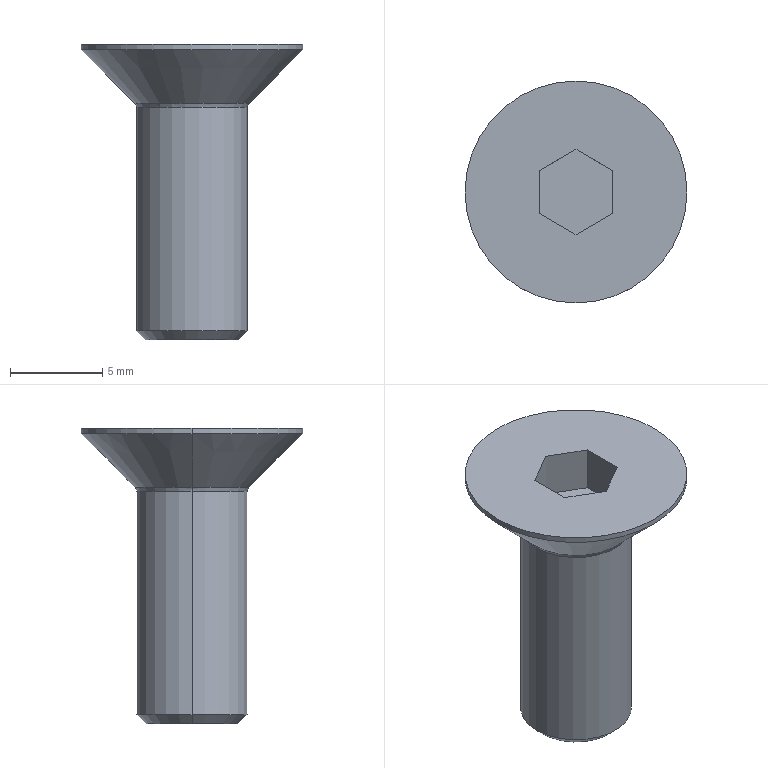Part | STEP file | DIN 7991 - M6x16 | 1 solid | 19 faces | box 12 x 12 x 16 mm | volume 554.104 mm3 | plane 9 | cylinder 4 | cone 4 | spline 2 | commonest cylinder face diameters 6 x2 12 x2
STEP:
#1=CARTESIAN_POINT('',(0.,0.,0.));
#2=DIRECTION('',(0.,0.,1.));
#3=DIRECTION('',(1.,0.,0.));
#4=AXIS2_PLACEMENT_3D('',#1,#2,#3);
#5=CARTESIAN_POINT('',(-3.088,0.,-3.212));
#6=VERTEX_POINT('',#5);
#7=CARTESIAN_POINT('',(-3.,0.,-3.424));
#8=VERTEX_POINT('',#7);
#9=CARTESIAN_POINT('',(-3.3,0.,-3.424));
#10=DIRECTION('',(0.,1.,0.));
#11=DIRECTION('',(-1.,0.,0.));
#12=AXIS2_PLACEMENT_3D('',#9,#10,#11);
#13=CIRCLE('',#12,0.3);
#14=CARTESIAN_POINT('',(-3.088,0.,-3.212));
#15=CARTESIAN_POINT('',(-3.088,6.176,-3.212));
#16=CARTESIAN_POINT('',(3.088,6.176,-3.212));
#17=CARTESIAN_POINT('',(3.088,0.,-3.212));
#18=CARTESIAN_POINT('',(-3.031,0.,-3.269));
#19=CARTESIAN_POINT('',(-3.031,6.062,-3.269));
#20=CARTESIAN_POINT('',(3.031,6.062,-3.269));
#21=CARTESIAN_POINT('',(3.031,0.,-3.269));
#22=CARTESIAN_POINT('',(-3.,0.,-3.344));
#23=CARTESIAN_POINT('',(-3.,6.,-3.344));
#24=CARTESIAN_POINT('',(3.,6.,-3.344));
#25=CARTESIAN_POINT('',(3.,0.,-3.344));
#26=CARTESIAN_POINT('',(-3.,0.,-3.424));
#27=CARTESIAN_POINT('',(-3.,6.,-3.424));
#28=CARTESIAN_POINT('',(3.,6.,-3.424));
#29=CARTESIAN_POINT('',(3.,0.,-3.424));
#30=(BOUNDED_SURFACE()B_SPLINE_SURFACE(3,3,((#14,#15,#16,#17),(#18,#19,#20,#21),(#22,#23,#24,#25),(#26,#27,#28,#29)),.UNSPECIFIED.,.F.,.F.,.F.)B_SPLINE_SURFACE_WITH_KNOTS((4,4),(4,4),(0.,1.),(0.,1.),.PIECEWISE_BEZIER_KNOTS.)GEOMETRIC_REPRESENTATION_ITEM()RATIONAL_B_SPLINE_SURFACE(((1.,0.3333,0.3333,1.),(0.9493,0.3164,0.3164,0.9493),(0.9493,0.3164,0.3164,0.9493),(1.,0.3333,0.3333,1.)))REPRESENTATION_ITEM('')SURFACE());
#31=CARTESIAN_POINT('',(0.,0.));
#32=CARTESIAN_POINT('',(0.01555,0.));
#33=CARTESIAN_POINT('',(0.04653,0.));
#34=CARTESIAN_POINT('',(0.09271,0.));
#35=CARTESIAN_POINT('',(0.1386,0.));
#36=CARTESIAN_POINT('',(0.1843,0.));
#37=CARTESIAN_POINT('',(0.2298,0.));
#38=CARTESIAN_POINT('',(0.2751,0.));
#39=CARTESIAN_POINT('',(0.3202,0.));
#40=CARTESIAN_POINT('',(0.3653,0.));
#41=CARTESIAN_POINT('',(0.4102,0.));
#42=CARTESIAN_POINT('',(0.4551,0.));
#43=CARTESIAN_POINT('',(0.5,0.));
#44=CARTESIAN_POINT('',(0.5449,0.));
#45=CARTESIAN_POINT('',(0.5898,0.));
#46=CARTESIAN_POINT('',(0.6347,0.));
#47=CARTESIAN_POINT('',(0.6798,0.));
#48=CARTESIAN_POINT('',(0.7249,0.));
#49=CARTESIAN_POINT('',(0.7702,0.));
#50=CARTESIAN_POINT('',(0.8157,0.));
#51=CARTESIAN_POINT('',(0.8614,0.));
#52=CARTESIAN_POINT('',(0.9073,0.));
#53=CARTESIAN_POINT('',(0.9535,0.));
#54=CARTESIAN_POINT('',(0.9845,0.));
#55=CARTESIAN_POINT('',(1.,0.));
#56=B_SPLINE_CURVE_WITH_KNOTS('',3,(#31,#32,#33,#34,#35,#36,#37,#38,#39,#40,#41,#42,#43,#44,#45,#46,#47,#48,#49,#50,#51,#52,#53,#54,#55),.UNSPECIFIED.,.F.,.F.,(4,1,1,1,1,1,1,1,1,1,1,1,1,1,1,1,1,1,1,1,1,1,4),(2.356,2.392,2.428,2.463,2.499,2.535,2.57,2.606,2.642,2.677,2.713,2.749,2.785,2.82,2.856,2.892,2.927,2.963,2.999,3.034,3.07,3.106,3.142),.QUASI_UNIFORM_KNOTS.);
#57=(GEOMETRIC_REPRESENTATION_CONTEXT(2)PARAMETRIC_REPRESENTATION_CONTEXT()REPRESENTATION_CONTEXT('',''));
#58=DEFINITIONAL_REPRESENTATION('',(#56),#57);
#59=PCURVE('',#30,#58);
#60=CARTESIAN_POINT('',(3.088,0.,-3.212));
#61=CARTESIAN_POINT('',(3.088,-6.176,-3.212));
#62=CARTESIAN_POINT('',(-3.088,-6.176,-3.212));
#63=CARTESIAN_POINT('',(-3.088,0.,-3.212));
#64=CARTESIAN_POINT('',(3.031,0.,-3.269));
#65=CARTESIAN_POINT('',(3.031,-6.062,-3.269));
#66=CARTESIAN_POINT('',(-3.031,-6.062,-3.269));
#67=CARTESIAN_POINT('',(-3.031,0.,-3.269));
#68=CARTESIAN_POINT('',(3.,0.,-3.344));
#69=CARTESIAN_POINT('',(3.,-6.,-3.344));
#70=CARTESIAN_POINT('',(-3.,-6.,-3.344));
#71=CARTESIAN_POINT('',(-3.,0.,-3.344));
#72=CARTESIAN_POINT('',(3.,0.,-3.424));
#73=CARTESIAN_POINT('',(3.,-6.,-3.424));
#74=CARTESIAN_POINT('',(-3.,-6.,-3.424));
#75=CARTESIAN_POINT('',(-3.,0.,-3.424));
#76=(BOUNDED_SURFACE()B_SPLINE_SURFACE(3,3,((#60,#61,#62,#63),(#64,#65,#66,#67),(#68,#69,#70,#71),(#72,#73,#74,#75)),.UNSPECIFIED.,.F.,.F.,.F.)B_SPLINE_SURFACE_WITH_KNOTS((4,4),(4,4),(0.,1.),(0.,1.),.PIECEWISE_BEZIER_KNOTS.)GEOMETRIC_REPRESENTATION_ITEM()RATIONAL_B_SPLINE_SURFACE(((1.,0.3333,0.3333,1.),(0.9493,0.3164,0.3164,0.9493),(0.9493,0.3164,0.3164,0.9493),(1.,0.3333,0.3333,1.)))REPRESENTATION_ITEM('')SURFACE());
#77=CARTESIAN_POINT('',(0.,1.));
#78=CARTESIAN_POINT('',(0.01555,1.));
#79=CARTESIAN_POINT('',(0.04653,1.));
#80=CARTESIAN_POINT('',(0.09271,1.));
#81=CARTESIAN_POINT('',(0.1386,1.));
#82=CARTESIAN_POINT('',(0.1843,1.));
#83=CARTESIAN_POINT('',(0.2298,1.));
#84=CARTESIAN_POINT('',(0.2751,1.));
#85=CARTESIAN_POINT('',(0.3202,1.));
#86=CARTESIAN_POINT('',(0.3653,1.));
#87=CARTESIAN_POINT('',(0.4102,1.));
#88=CARTESIAN_POINT('',(0.4551,1.));
#89=CARTESIAN_POINT('',(0.5,1.));
#90=CARTESIAN_POINT('',(0.5449,1.));
#91=CARTESIAN_POINT('',(0.5898,1.));
#92=CARTESIAN_POINT('',(0.6347,1.));
#93=CARTESIAN_POINT('',(0.6798,1.));
#94=CARTESIAN_POINT('',(0.7249,1.));
#95=CARTESIAN_POINT('',(0.7702,1.));
#96=CARTESIAN_POINT('',(0.8157,1.));
#97=CARTESIAN_POINT('',(0.8614,1.));
#98=CARTESIAN_POINT('',(0.9073,1.));
#99=CARTESIAN_POINT('',(0.9535,1.));
#100=CARTESIAN_POINT('',(0.9845,1.));
#101=CARTESIAN_POINT('',(1.,1.));
#102=B_SPLINE_CURVE_WITH_KNOTS('',3,(#77,#78,#79,#80,#81,#82,#83,#84,#85,#86,#87,#88,#89,#90,#91,#92,#93,#94,#95,#96,#97,#98,#99,#100,#101),.UNSPECIFIED.,.F.,.F.,(4,1,1,1,1,1,1,1,1,1,1,1,1,1,1,1,1,1,1,1,1,1,4),(2.356,2.392,2.428,2.463,2.499,2.535,2.57,2.606,2.642,2.677,2.713,2.749,2.785,2.82,2.856,2.892,2.927,2.963,2.999,3.034,3.07,3.106,3.142),.QUASI_UNIFORM_KNOTS.);
#103=(GEOMETRIC_REPRESENTATION_CONTEXT(2)PARAMETRIC_REPRESENTATION_CONTEXT()REPRESENTATION_CONTEXT('',''));
#104=DEFINITIONAL_REPRESENTATION('',(#102),#103);
#105=PCURVE('',#76,#104);
#106=SURFACE_CURVE('',#13,(#59,#105),.PCURVE_S1.);
#107=EDGE_CURVE('',#6,#8,#106,.T.);
#108=ORIENTED_EDGE('',*,*,#107,.T.);
#109=CARTESIAN_POINT('',(3.,0.,-3.424));
#110=VERTEX_POINT('',#109);
#111=CARTESIAN_POINT('',(0.,0.,-3.424));
#112=DIRECTION('',(0.,0.,-1.));
#113=DIRECTION('',(-1.,0.,0.));
#114=AXIS2_PLACEMENT_3D('',#111,#112,#113);
#115=CIRCLE('',#114,3.);
#116=CARTESIAN_POINT('',(1.,0.));
#117=CARTESIAN_POINT('',(1.,0.02375));
#118=CARTESIAN_POINT('',(1.,0.06805));
#119=CARTESIAN_POINT('',(1.,0.1267));
#120=CARTESIAN_POINT('',(1.,0.1794));
#121=CARTESIAN_POINT('',(1.,0.2276));
#122=CARTESIAN_POINT('',(1.,0.2721));
#123=CARTESIAN_POINT('',(1.,0.3139));
#124=CARTESIAN_POINT('',(1.,0.3535));
#125=CARTESIAN_POINT('',(1.,0.3914));
#126=CARTESIAN_POINT('',(1.,0.4282));
#127=CARTESIAN_POINT('',(1.,0.4643));
#128=CARTESIAN_POINT('',(1.,0.5));
#129=CARTESIAN_POINT('',(1.,0.5357));
#130=CARTESIAN_POINT('',(1.,0.5718));
#131=CARTESIAN_POINT('',(1.,0.6086));
#132=CARTESIAN_POINT('',(1.,0.6465));
#133=CARTESIAN_POINT('',(1.,0.6861));
#134=CARTESIAN_POINT('',(1.,0.7279));
#135=CARTESIAN_POINT('',(1.,0.7724));
#136=CARTESIAN_POINT('',(1.,0.8206));
#137=CARTESIAN_POINT('',(1.,0.8733));
#138=CARTESIAN_POINT('',(1.,0.9319));
#139=CARTESIAN_POINT('',(1.,0.9763));
#140=CARTESIAN_POINT('',(1.,1.));
#141=B_SPLINE_CURVE_WITH_KNOTS('',3,(#116,#117,#118,#119,#120,#121,#122,#123,#124,#125,#126,#127,#128,#129,#130,#131,#132,#133,#134,#135,#136,#137,#138,#139,#140),.UNSPECIFIED.,.F.,.F.,(4,1,1,1,1,1,1,1,1,1,1,1,1,1,1,1,1,1,1,1,1,1,4),(0.,0.1428,0.2856,0.4284,0.5712,0.714,0.8568,0.9996,1.142,1.285,1.428,1.571,1.714,1.856,1.999,2.142,2.285,2.428,2.57,2.713,2.856,2.999,3.142),.QUASI_UNIFORM_KNOTS.);
#142=(GEOMETRIC_REPRESENTATION_CONTEXT(2)PARAMETRIC_REPRESENTATION_CONTEXT()REPRESENTATION_CONTEXT('',''));
#143=DEFINITIONAL_REPRESENTATION('',(#141),#142);
#144=PCURVE('',#30,#143);
#145=CARTESIAN_POINT('',(0.,0.,-9.65));
#146=DIRECTION('',(0.,0.,-1.));
#147=DIRECTION('',(-1.,0.,0.));
#148=AXIS2_PLACEMENT_3D('',#145,#146,#147);
#149=CYLINDRICAL_SURFACE('',#148,3.);
#150=CARTESIAN_POINT('',(0.,-6.226));
#151=DIRECTION('',(1.,0.));
#152=VECTOR('',#151,1.);
#153=LINE('',#150,#152);
#154=(GEOMETRIC_REPRESENTATION_CONTEXT(2)PARAMETRIC_REPRESENTATION_CONTEXT()REPRESENTATION_CONTEXT('',''));
#155=DEFINITIONAL_REPRESENTATION('',(#153),#154);
#156=PCURVE('',#149,#155);
#157=SURFACE_CURVE('',#115,(#144,#156),.PCURVE_S1.);
#158=EDGE_CURVE('',#8,#110,#157,.T.);
#159=ORIENTED_EDGE('',*,*,#158,.T.);
#160=CARTESIAN_POINT('',(3.088,0.,-3.212));
#161=VERTEX_POINT('',#160);
#162=CARTESIAN_POINT('',(3.3,0.,-3.424));
#163=DIRECTION('',(0.,-1.,0.));
#164=DIRECTION('',(1.,0.,0.));
#165=AXIS2_PLACEMENT_3D('',#162,#163,#164);
#166=CIRCLE('',#165,0.3);
#167=CARTESIAN_POINT('',(0.,1.));
#168=CARTESIAN_POINT('',(0.01555,1.));
#169=CARTESIAN_POINT('',(0.04653,1.));
#170=CARTESIAN_POINT('',(0.09271,1.));
#171=CARTESIAN_POINT('',(0.1386,1.));
#172=CARTESIAN_POINT('',(0.1843,1.));
#173=CARTESIAN_POINT('',(0.2298,1.));
#174=CARTESIAN_POINT('',(0.2751,1.));
#175=CARTESIAN_POINT('',(0.3202,1.));
#176=CARTESIAN_POINT('',(0.3653,1.));
#177=CARTESIAN_POINT('',(0.4102,1.));
#178=CARTESIAN_POINT('',(0.4551,1.));
#179=CARTESIAN_POINT('',(0.5,1.));
#180=CARTESIAN_POINT('',(0.5449,1.));
#181=CARTESIAN_POINT('',(0.5898,1.));
#182=CARTESIAN_POINT('',(0.6347,1.));
#183=CARTESIAN_POINT('',(0.6798,1.));
#184=CARTESIAN_POINT('',(0.7249,1.));
#185=CARTESIAN_POINT('',(0.7702,1.));
#186=CARTESIAN_POINT('',(0.8157,1.));
#187=CARTESIAN_POINT('',(0.8614,1.));
#188=CARTESIAN_POINT('',(0.9073,1.));
#189=CARTESIAN_POINT('',(0.9535,1.));
#190=CARTESIAN_POINT('',(0.9845,1.));
#191=CARTESIAN_POINT('',(1.,1.));
#192=B_SPLINE_CURVE_WITH_KNOTS('',3,(#167,#168,#169,#170,#171,#172,#173,#174,#175,#176,#177,#178,#179,#180,#181,#182,#183,#184,#185,#186,#187,#188,#189,#190,#191),.UNSPECIFIED.,.F.,.F.,(4,1,1,1,1,1,1,1,1,1,1,1,1,1,1,1,1,1,1,1,1,1,4),(2.356,2.392,2.428,2.463,2.499,2.535,2.57,2.606,2.642,2.677,2.713,2.749,2.785,2.82,2.856,2.892,2.927,2.963,2.999,3.034,3.07,3.106,3.142),.QUASI_UNIFORM_KNOTS.);
#193=(GEOMETRIC_REPRESENTATION_CONTEXT(2)PARAMETRIC_REPRESENTATION_CONTEXT()REPRESENTATION_CONTEXT('',''));
#194=DEFINITIONAL_REPRESENTATION('',(#192),#193);
#195=PCURVE('',#30,#194);
#196=CARTESIAN_POINT('',(0.,0.));
#197=CARTESIAN_POINT('',(0.01555,0.));
#198=CARTESIAN_POINT('',(0.04653,0.));
#199=CARTESIAN_POINT('',(0.09271,0.));
#200=CARTESIAN_POINT('',(0.1386,0.));
#201=CARTESIAN_POINT('',(0.1843,0.));
#202=CARTESIAN_POINT('',(0.2298,0.));
#203=CARTESIAN_POINT('',(0.2751,0.));
#204=CARTESIAN_POINT('',(0.3202,0.));
#205=CARTESIAN_POINT('',(0.3653,0.));
#206=CARTESIAN_POINT('',(0.4102,0.));
#207=CARTESIAN_POINT('',(0.4551,0.));
#208=CARTESIAN_POINT('',(0.5,0.));
#209=CARTESIAN_POINT('',(0.5449,0.));
#210=CARTESIAN_POINT('',(0.5898,0.));
#211=CARTESIAN_POINT('',(0.6347,0.));
#212=CARTESIAN_POINT('',(0.6798,0.));
#213=CARTESIAN_POINT('',(0.7249,0.));
#214=CARTESIAN_POINT('',(0.7702,0.));
#215=CARTESIAN_POINT('',(0.8157,0.));
#216=CARTESIAN_POINT('',(0.8614,0.));
#217=CARTESIAN_POINT('',(0.9073,0.));
#218=CARTESIAN_POINT('',(0.9535,0.));
#219=CARTESIAN_POINT('',(0.9845,0.));
#220=CARTESIAN_POINT('',(1.,0.));
#221=B_SPLINE_CURVE_WITH_KNOTS('',3,(#196,#197,#198,#199,#200,#201,#202,#203,#204,#205,#206,#207,#208,#209,#210,#211,#212,#213,#214,#215,#216,#217,#218,#219,#220),.UNSPECIFIED.,.F.,.F.,(4,1,1,1,1,1,1,1,1,1,1,1,1,1,1,1,1,1,1,1,1,1,4),(2.356,2.392,2.428,2.463,2.499,2.535,2.57,2.606,2.642,2.677,2.713,2.749,2.785,2.82,2.856,2.892,2.927,2.963,2.999,3.034,3.07,3.106,3.142),.QUASI_UNIFORM_KNOTS.);
#222=(GEOMETRIC_REPRESENTATION_CONTEXT(2)PARAMETRIC_REPRESENTATION_CONTEXT()REPRESENTATION_CONTEXT('',''));
#223=DEFINITIONAL_REPRESENTATION('',(#221),#222);
#224=PCURVE('',#76,#223);
#225=SURFACE_CURVE('',#166,(#195,#224),.PCURVE_S1.);
#226=EDGE_CURVE('',#161,#110,#225,.T.);
#227=ORIENTED_EDGE('',*,*,#226,.F.);
#228=CARTESIAN_POINT('',(0.,0.,-3.212));
#229=DIRECTION('',(0.,0.,1.));
#230=DIRECTION('',(-1.,0.,0.));
#231=AXIS2_PLACEMENT_3D('',#228,#229,#230);
#232=CIRCLE('',#231,3.088);
#233=CARTESIAN_POINT('',(0.,1.));
#234=CARTESIAN_POINT('',(0.,0.9763));
#235=CARTESIAN_POINT('',(0.,0.9319));
#236=CARTESIAN_POINT('',(0.,0.8733));
#237=CARTESIAN_POINT('',(0.,0.8206));
#238=CARTESIAN_POINT('',(0.,0.7724));
#239=CARTESIAN_POINT('',(0.,0.7279));
#240=CARTESIAN_POINT('',(0.,0.6861));
#241=CARTESIAN_POINT('',(0.,0.6465));
#242=CARTESIAN_POINT('',(0.,0.6086));
#243=CARTESIAN_POINT('',(0.,0.5718));
#244=CARTESIAN_POINT('',(0.,0.5357));
#245=CARTESIAN_POINT('',(0.,0.5));
#246=CARTESIAN_POINT('',(0.,0.4643));
#247=CARTESIAN_POINT('',(0.,0.4282));
#248=CARTESIAN_POINT('',(0.,0.3914));
#249=CARTESIAN_POINT('',(0.,0.3535));
#250=CARTESIAN_POINT('',(0.,0.3139));
#251=CARTESIAN_POINT('',(0.,0.2721));
#252=CARTESIAN_POINT('',(0.,0.2276));
#253=CARTESIAN_POINT('',(0.,0.1794));
#254=CARTESIAN_POINT('',(0.,0.1267));
#255=CARTESIAN_POINT('',(0.,0.06805));
#256=CARTESIAN_POINT('',(0.,0.02375));
#257=CARTESIAN_POINT('',(0.,0.));
#258=B_SPLINE_CURVE_WITH_KNOTS('',3,(#233,#234,#235,#236,#237,#238,#239,#240,#241,#242,#243,#244,#245,#246,#247,#248,#249,#250,#251,#252,#253,#254,#255,#256,#257),.UNSPECIFIED.,.F.,.F.,(4,1,1,1,1,1,1,1,1,1,1,1,1,1,1,1,1,1,1,1,1,1,4),(3.142,3.284,3.427,3.57,3.713,3.856,3.998,4.141,4.284,4.427,4.57,4.712,4.855,4.998,5.141,5.284,5.426,5.569,5.712,5.855,5.998,6.14,6.283),.QUASI_UNIFORM_KNOTS.);
#259=(GEOMETRIC_REPRESENTATION_CONTEXT(2)PARAMETRIC_REPRESENTATION_CONTEXT()REPRESENTATION_CONTEXT('',''));
#260=DEFINITIONAL_REPRESENTATION('',(#258),#259);
#261=PCURVE('',#30,#260);
#262=CARTESIAN_POINT('',(0.,0.,-0.3));
#263=DIRECTION('',(0.,0.,1.));
#264=DIRECTION('',(1.,0.,0.));
#265=AXIS2_PLACEMENT_3D('',#262,#263,#264);
#266=CONICAL_SURFACE('',#265,6.,0.7854);
#267=CARTESIAN_POINT('',(-3.142,-2.912));
#268=DIRECTION('',(1.,0.));
#269=VECTOR('',#268,1.);
#270=LINE('',#267,#269);
#271=(GEOMETRIC_REPRESENTATION_CONTEXT(2)PARAMETRIC_REPRESENTATION_CONTEXT()REPRESENTATION_CONTEXT('',''));
#272=DEFINITIONAL_REPRESENTATION('',(#270),#271);
#273=PCURVE('',#266,#272);
#274=SURFACE_CURVE('',#232,(#261,#273),.PCURVE_S1.);
#275=EDGE_CURVE('',#161,#6,#274,.T.);
#276=ORIENTED_EDGE('',*,*,#275,.T.);
#277=EDGE_LOOP('',(#108,#159,#227,#276));
#278=FACE_BOUND('',#277,.F.);
#279=ADVANCED_FACE('',(#278),#30,.F.);
#280=ORIENTED_EDGE('',*,*,#158,.T.);
#281=CARTESIAN_POINT('',(3.,0.,-15.5));
#282=VERTEX_POINT('',#281);
#283=CARTESIAN_POINT('',(3.,0.,-9.65));
#284=DIRECTION('',(0.,0.,-1.));
#285=VECTOR('',#284,1.);
#286=LINE('',#283,#285);
#287=CARTESIAN_POINT('',(3.142,0.));
#288=DIRECTION('',(0.,1.));
#289=VECTOR('',#288,1.);
#290=LINE('',#287,#289);
#291=(GEOMETRIC_REPRESENTATION_CONTEXT(2)PARAMETRIC_REPRESENTATION_CONTEXT()REPRESENTATION_CONTEXT('',''));
#292=DEFINITIONAL_REPRESENTATION('',(#290),#291);
#293=PCURVE('',#149,#292);
#294=CARTESIAN_POINT('',(0.,0.,-9.65));
#295=DIRECTION('',(0.,0.,-1.));
#296=DIRECTION('',(-1.,0.,0.));
#297=AXIS2_PLACEMENT_3D('',#294,#295,#296);
#298=CYLINDRICAL_SURFACE('',#297,3.);
#299=CARTESIAN_POINT('',(3.142,0.));
#300=DIRECTION('',(0.,1.));
#301=VECTOR('',#300,1.);
#302=LINE('',#299,#301);
#303=(GEOMETRIC_REPRESENTATION_CONTEXT(2)PARAMETRIC_REPRESENTATION_CONTEXT()REPRESENTATION_CONTEXT('',''));
#304=DEFINITIONAL_REPRESENTATION('',(#302),#303);
#305=PCURVE('',#298,#304);
#306=SURFACE_CURVE('',#286,(#293,#305),.PCURVE_S1.);
#307=EDGE_CURVE('',#110,#282,#306,.T.);
#308=ORIENTED_EDGE('',*,*,#307,.T.);
#309=CARTESIAN_POINT('',(-3.,0.,-15.5));
#310=VERTEX_POINT('',#309);
#311=CARTESIAN_POINT('',(0.,0.,-15.5));
#312=DIRECTION('',(0.,0.,1.));
#313=DIRECTION('',(-1.,0.,0.));
#314=AXIS2_PLACEMENT_3D('',#311,#312,#313);
#315=CIRCLE('',#314,3.);
#316=CARTESIAN_POINT('',(6.283,5.85));
#317=DIRECTION('',(-1.,0.));
#318=VECTOR('',#317,1.);
#319=LINE('',#316,#318);
#320=(GEOMETRIC_REPRESENTATION_CONTEXT(2)PARAMETRIC_REPRESENTATION_CONTEXT()REPRESENTATION_CONTEXT('',''));
#321=DEFINITIONAL_REPRESENTATION('',(#319),#320);
#322=PCURVE('',#149,#321);
#323=CARTESIAN_POINT('',(0.,0.,-15.5));
#324=DIRECTION('',(0.,0.,1.));
#325=DIRECTION('',(1.,0.,0.));
#326=AXIS2_PLACEMENT_3D('',#323,#324,#325);
#327=CONICAL_SURFACE('',#326,3.,0.7854);
#328=CARTESIAN_POINT('',(-3.142,0.));
#329=DIRECTION('',(1.,0.));
#330=VECTOR('',#329,1.);
#331=LINE('',#328,#330);
#332=(GEOMETRIC_REPRESENTATION_CONTEXT(2)PARAMETRIC_REPRESENTATION_CONTEXT()REPRESENTATION_CONTEXT('',''));
#333=DEFINITIONAL_REPRESENTATION('',(#331),#332);
#334=PCURVE('',#327,#333);
#335=SURFACE_CURVE('',#315,(#322,#334),.PCURVE_S1.);
#336=EDGE_CURVE('',#282,#310,#335,.T.);
#337=ORIENTED_EDGE('',*,*,#336,.T.);
#338=CARTESIAN_POINT('',(-3.,0.,-9.65));
#339=DIRECTION('',(0.,0.,-1.));
#340=VECTOR('',#339,1.);
#341=LINE('',#338,#340);
#342=CARTESIAN_POINT('',(0.,0.));
#343=DIRECTION('',(0.,1.));
#344=VECTOR('',#343,1.);
#345=LINE('',#342,#344);
#346=(GEOMETRIC_REPRESENTATION_CONTEXT(2)PARAMETRIC_REPRESENTATION_CONTEXT()REPRESENTATION_CONTEXT('',''));
#347=DEFINITIONAL_REPRESENTATION('',(#345),#346);
#348=PCURVE('',#149,#347);
#349=CARTESIAN_POINT('',(6.283,0.));
#350=DIRECTION('',(0.,1.));
#351=VECTOR('',#350,1.);
#352=LINE('',#349,#351);
#353=(GEOMETRIC_REPRESENTATION_CONTEXT(2)PARAMETRIC_REPRESENTATION_CONTEXT()REPRESENTATION_CONTEXT('',''));
#354=DEFINITIONAL_REPRESENTATION('',(#352),#353);
#355=PCURVE('',#298,#354);
#356=SURFACE_CURVE('',#341,(#348,#355),.PCURVE_S1.);
#357=EDGE_CURVE('',#8,#310,#356,.T.);
#358=ORIENTED_EDGE('',*,*,#357,.F.);
#359=EDGE_LOOP('',(#280,#308,#337,#358));
#360=FACE_BOUND('',#359,.T.);
#361=ADVANCED_FACE('',(#360),#149,.T.);
#362=CARTESIAN_POINT('',(2.5,0.,-16.));
#363=VERTEX_POINT('',#362);
#364=CARTESIAN_POINT('',(-2.5,0.,-16.));
#365=VERTEX_POINT('',#364);
#366=CARTESIAN_POINT('',(0.,0.,-16.));
#367=DIRECTION('',(0.,0.,1.));
#368=DIRECTION('',(1.,0.,0.));
#369=AXIS2_PLACEMENT_3D('',#366,#367,#368);
#370=CIRCLE('',#369,2.5);
#371=CARTESIAN_POINT('',(0.,-0.5));
#372=DIRECTION('',(1.,0.));
#373=VECTOR('',#372,1.);
#374=LINE('',#371,#373);
#375=(GEOMETRIC_REPRESENTATION_CONTEXT(2)PARAMETRIC_REPRESENTATION_CONTEXT()REPRESENTATION_CONTEXT('',''));
#376=DEFINITIONAL_REPRESENTATION('',(#374),#375);
#377=PCURVE('',#327,#376);
#378=CARTESIAN_POINT('',(1.5,0.,-16.));
#379=DIRECTION('',(0.,0.,-1.));
#380=DIRECTION('',(-1.,0.,0.));
#381=AXIS2_PLACEMENT_3D('',#378,#379,#380);
#382=PLANE('',#381);
#383=CARTESIAN_POINT('',(-1.,0.));
#384=CARTESIAN_POINT('',(-1.,4.33));
#385=CARTESIAN_POINT('',(2.75,2.165));
#386=CARTESIAN_POINT('',(6.5,0.));
#387=CARTESIAN_POINT('',(2.75,-2.165));
#388=CARTESIAN_POINT('',(-1.,-4.33));
#389=CARTESIAN_POINT('',(-1.,0.));
#390=(BOUNDED_CURVE()B_SPLINE_CURVE(2,(#383,#384,#385,#386,#387,#388,#389),.UNSPECIFIED.,.T.,.F.)B_SPLINE_CURVE_WITH_KNOTS((1,2,2,2,2,1),(-2.094,0.,2.094,4.189,6.283,8.378),.UNSPECIFIED.)CURVE()GEOMETRIC_REPRESENTATION_ITEM()RATIONAL_B_SPLINE_CURVE((1.,0.5,1.,0.5,1.,0.5,1.))REPRESENTATION_ITEM(''));
#391=(GEOMETRIC_REPRESENTATION_CONTEXT(2)PARAMETRIC_REPRESENTATION_CONTEXT()REPRESENTATION_CONTEXT('',''));
#392=DEFINITIONAL_REPRESENTATION('',(#390),#391);
#393=PCURVE('',#382,#392);
#394=SURFACE_CURVE('',#370,(#377,#393),.PCURVE_S1.);
#395=EDGE_CURVE('',#363,#365,#394,.T.);
#396=ORIENTED_EDGE('',*,*,#395,.T.);
#397=CARTESIAN_POINT('',(-3.,0.,-15.5));
#398=DIRECTION('',(-0.7071,0.,0.7071));
#399=VECTOR('',#398,1.);
#400=LINE('',#397,#399);
#401=CARTESIAN_POINT('',(3.142,0.));
#402=DIRECTION('',(0.,1.));
#403=VECTOR('',#402,1.);
#404=LINE('',#401,#403);
#405=(GEOMETRIC_REPRESENTATION_CONTEXT(2)PARAMETRIC_REPRESENTATION_CONTEXT()REPRESENTATION_CONTEXT('',''));
#406=DEFINITIONAL_REPRESENTATION('',(#404),#405);
#407=PCURVE('',#327,#406);
#408=CARTESIAN_POINT('',(0.,0.,-15.5));
#409=DIRECTION('',(0.,0.,1.));
#410=DIRECTION('',(1.,0.,0.));
#411=AXIS2_PLACEMENT_3D('',#408,#409,#410);
#412=CONICAL_SURFACE('',#411,3.,0.7854);
#413=CARTESIAN_POINT('',(3.142,0.));
#414=DIRECTION('',(0.,1.));
#415=VECTOR('',#414,1.);
#416=LINE('',#413,#415);
#417=(GEOMETRIC_REPRESENTATION_CONTEXT(2)PARAMETRIC_REPRESENTATION_CONTEXT()REPRESENTATION_CONTEXT('',''));
#418=DEFINITIONAL_REPRESENTATION('',(#416),#417);
#419=PCURVE('',#412,#418);
#420=SURFACE_CURVE('',#400,(#407,#419),.PCURVE_S1.);
#421=EDGE_CURVE('',#365,#310,#420,.T.);
#422=ORIENTED_EDGE('',*,*,#421,.T.);
#423=ORIENTED_EDGE('',*,*,#336,.F.);
#424=CARTESIAN_POINT('',(3.,0.,-15.5));
#425=DIRECTION('',(0.7071,0.,0.7071));
#426=VECTOR('',#425,1.);
#427=LINE('',#424,#426);
#428=CARTESIAN_POINT('',(0.,0.));
#429=DIRECTION('',(0.,1.));
#430=VECTOR('',#429,1.);
#431=LINE('',#428,#430);
#432=(GEOMETRIC_REPRESENTATION_CONTEXT(2)PARAMETRIC_REPRESENTATION_CONTEXT()REPRESENTATION_CONTEXT('',''));
#433=DEFINITIONAL_REPRESENTATION('',(#431),#432);
#434=PCURVE('',#327,#433);
#435=CARTESIAN_POINT('',(6.283,0.));
#436=DIRECTION('',(0.,1.));
#437=VECTOR('',#436,1.);
#438=LINE('',#435,#437);
#439=(GEOMETRIC_REPRESENTATION_CONTEXT(2)PARAMETRIC_REPRESENTATION_CONTEXT()REPRESENTATION_CONTEXT('',''));
#440=DEFINITIONAL_REPRESENTATION('',(#438),#439);
#441=PCURVE('',#412,#440);
#442=SURFACE_CURVE('',#427,(#434,#441),.PCURVE_S1.);
#443=EDGE_CURVE('',#363,#282,#442,.T.);
#444=ORIENTED_EDGE('',*,*,#443,.F.);
#445=EDGE_LOOP('',(#396,#422,#423,#444));
#446=FACE_BOUND('',#445,.T.);
#447=ADVANCED_FACE('',(#446),#327,.T.);
#448=ORIENTED_EDGE('',*,*,#275,.T.);
#449=CARTESIAN_POINT('',(-6.,0.,-0.3));
#450=VERTEX_POINT('',#449);
#451=CARTESIAN_POINT('',(-6.,0.,-0.3));
#452=DIRECTION('',(-0.7071,0.,0.7071));
#453=VECTOR('',#452,1.);
#454=LINE('',#451,#453);
#455=CARTESIAN_POINT('',(3.142,0.));
#456=DIRECTION('',(0.,1.));
#457=VECTOR('',#456,1.);
#458=LINE('',#455,#457);
#459=(GEOMETRIC_REPRESENTATION_CONTEXT(2)PARAMETRIC_REPRESENTATION_CONTEXT()REPRESENTATION_CONTEXT('',''));
#460=DEFINITIONAL_REPRESENTATION('',(#458),#459);
#461=PCURVE('',#266,#460);
#462=CARTESIAN_POINT('',(0.,0.,-0.3));
#463=DIRECTION('',(0.,0.,1.));
#464=DIRECTION('',(1.,0.,0.));
#465=AXIS2_PLACEMENT_3D('',#462,#463,#464);
#466=CONICAL_SURFACE('',#465,6.,0.7854);
#467=CARTESIAN_POINT('',(3.142,0.));
#468=DIRECTION('',(0.,1.));
#469=VECTOR('',#468,1.);
#470=LINE('',#467,#469);
#471=(GEOMETRIC_REPRESENTATION_CONTEXT(2)PARAMETRIC_REPRESENTATION_CONTEXT()REPRESENTATION_CONTEXT('',''));
#472=DEFINITIONAL_REPRESENTATION('',(#470),#471);
#473=PCURVE('',#466,#472);
#474=SURFACE_CURVE('',#454,(#461,#473),.PCURVE_S1.);
#475=EDGE_CURVE('',#6,#450,#474,.T.);
#476=ORIENTED_EDGE('',*,*,#475,.T.);
#477=CARTESIAN_POINT('',(6.,0.,-0.3));
#478=VERTEX_POINT('',#477);
#479=CARTESIAN_POINT('',(0.,0.,-0.3));
#480=DIRECTION('',(0.,0.,-1.));
#481=DIRECTION('',(1.,0.,0.));
#482=AXIS2_PLACEMENT_3D('',#479,#480,#481);
#483=CIRCLE('',#482,6.);
#484=CARTESIAN_POINT('',(6.283,0.));
#485=DIRECTION('',(-1.,0.));
#486=VECTOR('',#485,1.);
#487=LINE('',#484,#486);
#488=(GEOMETRIC_REPRESENTATION_CONTEXT(2)PARAMETRIC_REPRESENTATION_CONTEXT()REPRESENTATION_CONTEXT('',''));
#489=DEFINITIONAL_REPRESENTATION('',(#487),#488);
#490=PCURVE('',#266,#489);
#491=CARTESIAN_POINT('',(0.,0.,-0.15));
#492=DIRECTION('',(0.,0.,-1.));
#493=DIRECTION('',(-1.,0.,0.));
#494=AXIS2_PLACEMENT_3D('',#491,#492,#493);
#495=CYLINDRICAL_SURFACE('',#494,6.);
#496=CARTESIAN_POINT('',(-3.142,0.15));
#497=DIRECTION('',(1.,0.));
#498=VECTOR('',#497,1.);
#499=LINE('',#496,#498);
#500=(GEOMETRIC_REPRESENTATION_CONTEXT(2)PARAMETRIC_REPRESENTATION_CONTEXT()REPRESENTATION_CONTEXT('',''));
#501=DEFINITIONAL_REPRESENTATION('',(#499),#500);
#502=PCURVE('',#495,#501);
#503=SURFACE_CURVE('',#483,(#490,#502),.PCURVE_S1.);
#504=EDGE_CURVE('',#450,#478,#503,.T.);
#505=ORIENTED_EDGE('',*,*,#504,.T.);
#506=CARTESIAN_POINT('',(6.,0.,-0.3));
#507=DIRECTION('',(0.7071,0.,0.7071));
#508=VECTOR('',#507,1.);
#509=LINE('',#506,#508);
#510=CARTESIAN_POINT('',(0.,0.));
#511=DIRECTION('',(0.,1.));
#512=VECTOR('',#511,1.);
#513=LINE('',#510,#512);
#514=(GEOMETRIC_REPRESENTATION_CONTEXT(2)PARAMETRIC_REPRESENTATION_CONTEXT()REPRESENTATION_CONTEXT('',''));
#515=DEFINITIONAL_REPRESENTATION('',(#513),#514);
#516=PCURVE('',#266,#515);
#517=CARTESIAN_POINT('',(6.283,0.));
#518=DIRECTION('',(0.,1.));
#519=VECTOR('',#518,1.);
#520=LINE('',#517,#519);
#521=(GEOMETRIC_REPRESENTATION_CONTEXT(2)PARAMETRIC_REPRESENTATION_CONTEXT()REPRESENTATION_CONTEXT('',''));
#522=DEFINITIONAL_REPRESENTATION('',(#520),#521);
#523=PCURVE('',#466,#522);
#524=SURFACE_CURVE('',#509,(#516,#523),.PCURVE_S1.);
#525=EDGE_CURVE('',#161,#478,#524,.T.);
#526=ORIENTED_EDGE('',*,*,#525,.F.);
#527=EDGE_LOOP('',(#448,#476,#505,#526));
#528=FACE_BOUND('',#527,.T.);
#529=ADVANCED_FACE('',(#528),#266,.T.);
#530=CARTESIAN_POINT('',(-6.,0.,0.));
#531=VERTEX_POINT('',#530);
#532=CARTESIAN_POINT('',(6.,0.,0.));
#533=VERTEX_POINT('',#532);
#534=CARTESIAN_POINT('',(0.,0.,0.));
#535=DIRECTION('',(0.,0.,-1.));
#536=DIRECTION('',(-1.,0.,0.));
#537=AXIS2_PLACEMENT_3D('',#534,#535,#536);
#538=CIRCLE('',#537,6.);
#539=CARTESIAN_POINT('',(0.,-0.15));
#540=DIRECTION('',(1.,0.));
#541=VECTOR('',#540,1.);
#542=LINE('',#539,#541);
#543=(GEOMETRIC_REPRESENTATION_CONTEXT(2)PARAMETRIC_REPRESENTATION_CONTEXT()REPRESENTATION_CONTEXT('',''));
#544=DEFINITIONAL_REPRESENTATION('',(#542),#543);
#545=PCURVE('',#495,#544);
#546=CARTESIAN_POINT('',(3.,0.,0.));
#547=DIRECTION('',(0.,0.,1.));
#548=DIRECTION('',(1.,0.,0.));
#549=AXIS2_PLACEMENT_3D('',#546,#547,#548);
#550=PLANE('',#549);
#551=CARTESIAN_POINT('',(-9.,0.));
#552=CARTESIAN_POINT('',(-9.,10.392));
#553=CARTESIAN_POINT('',(0.,5.196));
#554=CARTESIAN_POINT('',(9.,0.));
#555=CARTESIAN_POINT('',(0.,-5.196));
#556=CARTESIAN_POINT('',(-9.,-10.392));
#557=CARTESIAN_POINT('',(-9.,0.));
#558=(BOUNDED_CURVE()B_SPLINE_CURVE(2,(#551,#552,#553,#554,#555,#556,#557),.UNSPECIFIED.,.T.,.F.)B_SPLINE_CURVE_WITH_KNOTS((1,2,2,2,2,1),(-2.094,0.,2.094,4.189,6.283,8.378),.UNSPECIFIED.)CURVE()GEOMETRIC_REPRESENTATION_ITEM()RATIONAL_B_SPLINE_CURVE((1.,0.5,1.,0.5,1.,0.5,1.))REPRESENTATION_ITEM(''));
#559=(GEOMETRIC_REPRESENTATION_CONTEXT(2)PARAMETRIC_REPRESENTATION_CONTEXT()REPRESENTATION_CONTEXT('',''));
#560=DEFINITIONAL_REPRESENTATION('',(#558),#559);
#561=PCURVE('',#550,#560);
#562=SURFACE_CURVE('',#538,(#545,#561),.PCURVE_S1.);
#563=EDGE_CURVE('',#531,#533,#562,.T.);
#564=ORIENTED_EDGE('',*,*,#563,.T.);
#565=CARTESIAN_POINT('',(6.,0.,-0.15));
#566=DIRECTION('',(0.,0.,-1.));
#567=VECTOR('',#566,1.);
#568=LINE('',#565,#567);
#569=CARTESIAN_POINT('',(3.142,0.));
#570=DIRECTION('',(0.,1.));
#571=VECTOR('',#570,1.);
#572=LINE('',#569,#571);
#573=(GEOMETRIC_REPRESENTATION_CONTEXT(2)PARAMETRIC_REPRESENTATION_CONTEXT()REPRESENTATION_CONTEXT('',''));
#574=DEFINITIONAL_REPRESENTATION('',(#572),#573);
#575=PCURVE('',#495,#574);
#576=CARTESIAN_POINT('',(0.,0.,-0.15));
#577=DIRECTION('',(0.,0.,-1.));
#578=DIRECTION('',(-1.,0.,0.));
#579=AXIS2_PLACEMENT_3D('',#576,#577,#578);
#580=CYLINDRICAL_SURFACE('',#579,6.);
#581=CARTESIAN_POINT('',(3.142,0.));
#582=DIRECTION('',(0.,1.));
#583=VECTOR('',#582,1.);
#584=LINE('',#581,#583);
#585=(GEOMETRIC_REPRESENTATION_CONTEXT(2)PARAMETRIC_REPRESENTATION_CONTEXT()REPRESENTATION_CONTEXT('',''));
#586=DEFINITIONAL_REPRESENTATION('',(#584),#585);
#587=PCURVE('',#580,#586);
#588=SURFACE_CURVE('',#568,(#575,#587),.PCURVE_S1.);
#589=EDGE_CURVE('',#533,#478,#588,.T.);
#590=ORIENTED_EDGE('',*,*,#589,.T.);
#591=ORIENTED_EDGE('',*,*,#504,.F.);
#592=CARTESIAN_POINT('',(-6.,0.,-0.15));
#593=DIRECTION('',(0.,0.,-1.));
#594=VECTOR('',#593,1.);
#595=LINE('',#592,#594);
#596=CARTESIAN_POINT('',(0.,0.));
#597=DIRECTION('',(0.,1.));
#598=VECTOR('',#597,1.);
#599=LINE('',#596,#598);
#600=(GEOMETRIC_REPRESENTATION_CONTEXT(2)PARAMETRIC_REPRESENTATION_CONTEXT()REPRESENTATION_CONTEXT('',''));
#601=DEFINITIONAL_REPRESENTATION('',(#599),#600);
#602=PCURVE('',#495,#601);
#603=CARTESIAN_POINT('',(6.283,0.));
#604=DIRECTION('',(0.,1.));
#605=VECTOR('',#604,1.);
#606=LINE('',#603,#605);
#607=(GEOMETRIC_REPRESENTATION_CONTEXT(2)PARAMETRIC_REPRESENTATION_CONTEXT()REPRESENTATION_CONTEXT('',''));
#608=DEFINITIONAL_REPRESENTATION('',(#606),#607);
#609=PCURVE('',#580,#608);
#610=SURFACE_CURVE('',#595,(#602,#609),.PCURVE_S1.);
#611=EDGE_CURVE('',#531,#450,#610,.T.);
#612=ORIENTED_EDGE('',*,*,#611,.F.);
#613=EDGE_LOOP('',(#564,#590,#591,#612));
#614=FACE_BOUND('',#613,.T.);
#615=ADVANCED_FACE('',(#614),#495,.T.);
#616=ORIENTED_EDGE('',*,*,#307,.F.);
#617=CARTESIAN_POINT('',(0.,0.,-3.424));
#618=DIRECTION('',(0.,0.,-1.));
#619=DIRECTION('',(-1.,0.,0.));
#620=AXIS2_PLACEMENT_3D('',#617,#618,#619);
#621=CIRCLE('',#620,3.);
#622=CARTESIAN_POINT('',(0.,-6.226));
#623=DIRECTION('',(1.,0.));
#624=VECTOR('',#623,1.);
#625=LINE('',#622,#624);
#626=(GEOMETRIC_REPRESENTATION_CONTEXT(2)PARAMETRIC_REPRESENTATION_CONTEXT()REPRESENTATION_CONTEXT('',''));
#627=DEFINITIONAL_REPRESENTATION('',(#625),#626);
#628=PCURVE('',#298,#627);
#629=CARTESIAN_POINT('',(1.,0.));
#630=CARTESIAN_POINT('',(1.,0.02375));
#631=CARTESIAN_POINT('',(1.,0.06805));
#632=CARTESIAN_POINT('',(1.,0.1267));
#633=CARTESIAN_POINT('',(1.,0.1794));
#634=CARTESIAN_POINT('',(1.,0.2276));
#635=CARTESIAN_POINT('',(1.,0.2721));
#636=CARTESIAN_POINT('',(1.,0.3139));
#637=CARTESIAN_POINT('',(1.,0.3535));
#638=CARTESIAN_POINT('',(1.,0.3914));
#639=CARTESIAN_POINT('',(1.,0.4282));
#640=CARTESIAN_POINT('',(1.,0.4643));
#641=CARTESIAN_POINT('',(1.,0.5));
#642=CARTESIAN_POINT('',(1.,0.5357));
#643=CARTESIAN_POINT('',(1.,0.5718));
#644=CARTESIAN_POINT('',(1.,0.6086));
#645=CARTESIAN_POINT('',(1.,0.6465));
#646=CARTESIAN_POINT('',(1.,0.6861));
#647=CARTESIAN_POINT('',(1.,0.7279));
#648=CARTESIAN_POINT('',(1.,0.7724));
#649=CARTESIAN_POINT('',(1.,0.8206));
#650=CARTESIAN_POINT('',(1.,0.8733));
#651=CARTESIAN_POINT('',(1.,0.9319));
#652=CARTESIAN_POINT('',(1.,0.9763));
#653=CARTESIAN_POINT('',(1.,1.));
#654=B_SPLINE_CURVE_WITH_KNOTS('',3,(#629,#630,#631,#632,#633,#634,#635,#636,#637,#638,#639,#640,#641,#642,#643,#644,#645,#646,#647,#648,#649,#650,#651,#652,#653),.UNSPECIFIED.,.F.,.F.,(4,1,1,1,1,1,1,1,1,1,1,1,1,1,1,1,1,1,1,1,1,1,4),(3.142,3.284,3.427,3.57,3.713,3.856,3.998,4.141,4.284,4.427,4.57,4.712,4.855,4.998,5.141,5.284,5.426,5.569,5.712,5.855,5.998,6.14,6.283),.QUASI_UNIFORM_KNOTS.);
#655=(GEOMETRIC_REPRESENTATION_CONTEXT(2)PARAMETRIC_REPRESENTATION_CONTEXT()REPRESENTATION_CONTEXT('',''));
#656=DEFINITIONAL_REPRESENTATION('',(#654),#655);
#657=PCURVE('',#76,#656);
#658=SURFACE_CURVE('',#621,(#628,#657),.PCURVE_S1.);
#659=EDGE_CURVE('',#110,#8,#658,.T.);
#660=ORIENTED_EDGE('',*,*,#659,.T.);
#661=ORIENTED_EDGE('',*,*,#357,.T.);
#662=CARTESIAN_POINT('',(0.,0.,-15.5));
#663=DIRECTION('',(0.,0.,1.));
#664=DIRECTION('',(-1.,0.,0.));
#665=AXIS2_PLACEMENT_3D('',#662,#663,#664);
#666=CIRCLE('',#665,3.);
#667=CARTESIAN_POINT('',(6.283,5.85));
#668=DIRECTION('',(-1.,0.));
#669=VECTOR('',#668,1.);
#670=LINE('',#667,#669);
#671=(GEOMETRIC_REPRESENTATION_CONTEXT(2)PARAMETRIC_REPRESENTATION_CONTEXT()REPRESENTATION_CONTEXT('',''));
#672=DEFINITIONAL_REPRESENTATION('',(#670),#671);
#673=PCURVE('',#298,#672);
#674=CARTESIAN_POINT('',(3.142,0.));
#675=DIRECTION('',(1.,0.));
#676=VECTOR('',#675,1.);
#677=LINE('',#674,#676);
#678=(GEOMETRIC_REPRESENTATION_CONTEXT(2)PARAMETRIC_REPRESENTATION_CONTEXT()REPRESENTATION_CONTEXT('',''));
#679=DEFINITIONAL_REPRESENTATION('',(#677),#678);
#680=PCURVE('',#412,#679);
#681=SURFACE_CURVE('',#666,(#673,#680),.PCURVE_S1.);
#682=EDGE_CURVE('',#310,#282,#681,.T.);
#683=ORIENTED_EDGE('',*,*,#682,.T.);
#684=EDGE_LOOP('',(#616,#660,#661,#683));
#685=FACE_BOUND('',#684,.T.);
#686=ADVANCED_FACE('',(#685),#298,.T.);
#687=ORIENTED_EDGE('',*,*,#421,.F.);
#688=CARTESIAN_POINT('',(0.,0.,-16.));
#689=DIRECTION('',(0.,0.,1.));
#690=DIRECTION('',(1.,0.,0.));
#691=AXIS2_PLACEMENT_3D('',#688,#689,#690);
#692=CIRCLE('',#691,2.5);
#693=CARTESIAN_POINT('',(0.,-0.5));
#694=DIRECTION('',(1.,0.));
#695=VECTOR('',#694,1.);
#696=LINE('',#693,#695);
#697=(GEOMETRIC_REPRESENTATION_CONTEXT(2)PARAMETRIC_REPRESENTATION_CONTEXT()REPRESENTATION_CONTEXT('',''));
#698=DEFINITIONAL_REPRESENTATION('',(#696),#697);
#699=PCURVE('',#412,#698);
#700=CARTESIAN_POINT('',(-1.,0.));
#701=CARTESIAN_POINT('',(-1.,4.33));
#702=CARTESIAN_POINT('',(2.75,2.165));
#703=CARTESIAN_POINT('',(6.5,0.));
#704=CARTESIAN_POINT('',(2.75,-2.165));
#705=CARTESIAN_POINT('',(-1.,-4.33));
#706=CARTESIAN_POINT('',(-1.,0.));
#707=(BOUNDED_CURVE()B_SPLINE_CURVE(2,(#700,#701,#702,#703,#704,#705,#706),.UNSPECIFIED.,.T.,.F.)B_SPLINE_CURVE_WITH_KNOTS((1,2,2,2,2,1),(-2.094,0.,2.094,4.189,6.283,8.378),.UNSPECIFIED.)CURVE()GEOMETRIC_REPRESENTATION_ITEM()RATIONAL_B_SPLINE_CURVE((1.,0.5,1.,0.5,1.,0.5,1.))REPRESENTATION_ITEM(''));
#708=(GEOMETRIC_REPRESENTATION_CONTEXT(2)PARAMETRIC_REPRESENTATION_CONTEXT()REPRESENTATION_CONTEXT('',''));
#709=DEFINITIONAL_REPRESENTATION('',(#707),#708);
#710=PCURVE('',#382,#709);
#711=SURFACE_CURVE('',#692,(#699,#710),.PCURVE_S1.);
#712=EDGE_CURVE('',#365,#363,#711,.T.);
#713=ORIENTED_EDGE('',*,*,#712,.T.);
#714=ORIENTED_EDGE('',*,*,#443,.T.);
#715=ORIENTED_EDGE('',*,*,#682,.F.);
#716=EDGE_LOOP('',(#687,#713,#714,#715));
#717=FACE_BOUND('',#716,.T.);
#718=ADVANCED_FACE('',(#717),#412,.T.);
#719=ORIENTED_EDGE('',*,*,#659,.T.);
#720=ORIENTED_EDGE('',*,*,#107,.F.);
#721=CARTESIAN_POINT('',(0.,0.,-3.212));
#722=DIRECTION('',(0.,0.,1.));
#723=DIRECTION('',(-1.,0.,0.));
#724=AXIS2_PLACEMENT_3D('',#721,#722,#723);
#725=CIRCLE('',#724,3.088);
#726=CARTESIAN_POINT('',(0.,1.));
#727=CARTESIAN_POINT('',(0.,0.9763));
#728=CARTESIAN_POINT('',(0.,0.9319));
#729=CARTESIAN_POINT('',(0.,0.8733));
#730=CARTESIAN_POINT('',(0.,0.8206));
#731=CARTESIAN_POINT('',(0.,0.7724));
#732=CARTESIAN_POINT('',(0.,0.7279));
#733=CARTESIAN_POINT('',(0.,0.6861));
#734=CARTESIAN_POINT('',(0.,0.6465));
#735=CARTESIAN_POINT('',(0.,0.6086));
#736=CARTESIAN_POINT('',(0.,0.5718));
#737=CARTESIAN_POINT('',(0.,0.5357));
#738=CARTESIAN_POINT('',(0.,0.5));
#739=CARTESIAN_POINT('',(0.,0.4643));
#740=CARTESIAN_POINT('',(0.,0.4282));
#741=CARTESIAN_POINT('',(0.,0.3914));
#742=CARTESIAN_POINT('',(0.,0.3535));
#743=CARTESIAN_POINT('',(0.,0.3139));
#744=CARTESIAN_POINT('',(0.,0.2721));
#745=CARTESIAN_POINT('',(0.,0.2276));
#746=CARTESIAN_POINT('',(0.,0.1794));
#747=CARTESIAN_POINT('',(0.,0.1267));
#748=CARTESIAN_POINT('',(0.,0.06805));
#749=CARTESIAN_POINT('',(0.,0.02375));
#750=CARTESIAN_POINT('',(0.,0.));
#751=B_SPLINE_CURVE_WITH_KNOTS('',3,(#726,#727,#728,#729,#730,#731,#732,#733,#734,#735,#736,#737,#738,#739,#740,#741,#742,#743,#744,#745,#746,#747,#748,#749,#750),.UNSPECIFIED.,.F.,.F.,(4,1,1,1,1,1,1,1,1,1,1,1,1,1,1,1,1,1,1,1,1,1,4),(0.,0.1428,0.2856,0.4284,0.5712,0.714,0.8568,0.9996,1.142,1.285,1.428,1.571,1.714,1.856,1.999,2.142,2.285,2.428,2.57,2.713,2.856,2.999,3.142),.QUASI_UNIFORM_KNOTS.);
#752=(GEOMETRIC_REPRESENTATION_CONTEXT(2)PARAMETRIC_REPRESENTATION_CONTEXT()REPRESENTATION_CONTEXT('',''));
#753=DEFINITIONAL_REPRESENTATION('',(#751),#752);
#754=PCURVE('',#76,#753);
#755=CARTESIAN_POINT('',(3.142,-2.912));
#756=DIRECTION('',(1.,0.));
#757=VECTOR('',#756,1.);
#758=LINE('',#755,#757);
#759=(GEOMETRIC_REPRESENTATION_CONTEXT(2)PARAMETRIC_REPRESENTATION_CONTEXT()REPRESENTATION_CONTEXT('',''));
#760=DEFINITIONAL_REPRESENTATION('',(#758),#759);
#761=PCURVE('',#466,#760);
#762=SURFACE_CURVE('',#725,(#754,#761),.PCURVE_S1.);
#763=EDGE_CURVE('',#6,#161,#762,.T.);
#764=ORIENTED_EDGE('',*,*,#763,.T.);
#765=ORIENTED_EDGE('',*,*,#226,.T.);
#766=EDGE_LOOP('',(#719,#720,#764,#765));
#767=FACE_BOUND('',#766,.F.);
#768=ADVANCED_FACE('',(#767),#76,.F.);
#769=ORIENTED_EDGE('',*,*,#395,.F.);
#770=ORIENTED_EDGE('',*,*,#712,.F.);
#771=EDGE_LOOP('',(#769,#770));
#772=FACE_BOUND('',#771,.T.);
#773=ADVANCED_FACE('',(#772),#382,.T.);
#774=ORIENTED_EDGE('',*,*,#475,.F.);
#775=ORIENTED_EDGE('',*,*,#763,.T.);
#776=ORIENTED_EDGE('',*,*,#525,.T.);
#777=CARTESIAN_POINT('',(0.,0.,-0.3));
#778=DIRECTION('',(0.,0.,-1.));
#779=DIRECTION('',(1.,0.,0.));
#780=AXIS2_PLACEMENT_3D('',#777,#778,#779);
#781=CIRCLE('',#780,6.);
#782=CARTESIAN_POINT('',(6.283,0.));
#783=DIRECTION('',(-1.,0.));
#784=VECTOR('',#783,1.);
#785=LINE('',#782,#784);
#786=(GEOMETRIC_REPRESENTATION_CONTEXT(2)PARAMETRIC_REPRESENTATION_CONTEXT()REPRESENTATION_CONTEXT('',''));
#787=DEFINITIONAL_REPRESENTATION('',(#785),#786);
#788=PCURVE('',#466,#787);
#789=CARTESIAN_POINT('',(3.142,0.15));
#790=DIRECTION('',(1.,0.));
#791=VECTOR('',#790,1.);
#792=LINE('',#789,#791);
#793=(GEOMETRIC_REPRESENTATION_CONTEXT(2)PARAMETRIC_REPRESENTATION_CONTEXT()REPRESENTATION_CONTEXT('',''));
#794=DEFINITIONAL_REPRESENTATION('',(#792),#793);
#795=PCURVE('',#580,#794);
#796=SURFACE_CURVE('',#781,(#788,#795),.PCURVE_S1.);
#797=EDGE_CURVE('',#478,#450,#796,.T.);
#798=ORIENTED_EDGE('',*,*,#797,.T.);
#799=EDGE_LOOP('',(#774,#775,#776,#798));
#800=FACE_BOUND('',#799,.T.);
#801=ADVANCED_FACE('',(#800),#466,.T.);
#802=ORIENTED_EDGE('',*,*,#589,.F.);
#803=CARTESIAN_POINT('',(0.,0.,0.));
#804=DIRECTION('',(0.,0.,-1.));
#805=DIRECTION('',(-1.,0.,0.));
#806=AXIS2_PLACEMENT_3D('',#803,#804,#805);
#807=CIRCLE('',#806,6.);
#808=CARTESIAN_POINT('',(0.,-0.15));
#809=DIRECTION('',(1.,0.));
#810=VECTOR('',#809,1.);
#811=LINE('',#808,#810);
#812=(GEOMETRIC_REPRESENTATION_CONTEXT(2)PARAMETRIC_REPRESENTATION_CONTEXT()REPRESENTATION_CONTEXT('',''));
#813=DEFINITIONAL_REPRESENTATION('',(#811),#812);
#814=PCURVE('',#580,#813);
#815=CARTESIAN_POINT('',(-9.,0.));
#816=CARTESIAN_POINT('',(-9.,10.392));
#817=CARTESIAN_POINT('',(0.,5.196));
#818=CARTESIAN_POINT('',(9.,0.));
#819=CARTESIAN_POINT('',(0.,-5.196));
#820=CARTESIAN_POINT('',(-9.,-10.392));
#821=CARTESIAN_POINT('',(-9.,0.));
#822=(BOUNDED_CURVE()B_SPLINE_CURVE(2,(#815,#816,#817,#818,#819,#820,#821),.UNSPECIFIED.,.T.,.F.)B_SPLINE_CURVE_WITH_KNOTS((1,2,2,2,2,1),(-2.094,0.,2.094,4.189,6.283,8.378),.UNSPECIFIED.)CURVE()GEOMETRIC_REPRESENTATION_ITEM()RATIONAL_B_SPLINE_CURVE((1.,0.5,1.,0.5,1.,0.5,1.))REPRESENTATION_ITEM(''));
#823=(GEOMETRIC_REPRESENTATION_CONTEXT(2)PARAMETRIC_REPRESENTATION_CONTEXT()REPRESENTATION_CONTEXT('',''));
#824=DEFINITIONAL_REPRESENTATION('',(#822),#823);
#825=PCURVE('',#550,#824);
#826=SURFACE_CURVE('',#807,(#814,#825),.PCURVE_S1.);
#827=EDGE_CURVE('',#533,#531,#826,.T.);
#828=ORIENTED_EDGE('',*,*,#827,.T.);
#829=ORIENTED_EDGE('',*,*,#611,.T.);
#830=ORIENTED_EDGE('',*,*,#797,.F.);
#831=EDGE_LOOP('',(#802,#828,#829,#830));
#832=FACE_BOUND('',#831,.T.);
#833=ADVANCED_FACE('',(#832),#580,.T.);
#834=CARTESIAN_POINT('',(2.,1.155,0.));
#835=VERTEX_POINT('',#834);
#836=CARTESIAN_POINT('',(2.,-1.155,0.));
#837=VERTEX_POINT('',#836);
#838=CARTESIAN_POINT('',(2.,0.,0.));
#839=DIRECTION('',(0.,-1.,0.));
#840=VECTOR('',#839,1.);
#841=LINE('',#838,#840);
#842=CARTESIAN_POINT('',(-1.,0.));
#843=DIRECTION('',(0.,-1.));
#844=VECTOR('',#843,1.);
#845=LINE('',#842,#844);
#846=(GEOMETRIC_REPRESENTATION_CONTEXT(2)PARAMETRIC_REPRESENTATION_CONTEXT()REPRESENTATION_CONTEXT('',''));
#847=DEFINITIONAL_REPRESENTATION('',(#845),#846);
#848=PCURVE('',#550,#847);
#849=CARTESIAN_POINT('',(2.,-1.155,0.));
#850=DIRECTION('',(1.,0.,0.));
#851=DIRECTION('',(0.,0.,-1.));
#852=AXIS2_PLACEMENT_3D('',#849,#850,#851);
#853=PLANE('',#852);
#854=CARTESIAN_POINT('',(0.,1.155));
#855=DIRECTION('',(0.,-1.));
#856=VECTOR('',#855,1.);
#857=LINE('',#854,#856);
#858=(GEOMETRIC_REPRESENTATION_CONTEXT(2)PARAMETRIC_REPRESENTATION_CONTEXT()REPRESENTATION_CONTEXT('',''));
#859=DEFINITIONAL_REPRESENTATION('',(#857),#858);
#860=PCURVE('',#853,#859);
#861=SURFACE_CURVE('',#841,(#848,#860),.PCURVE_S1.);
#862=EDGE_CURVE('',#835,#837,#861,.T.);
#863=ORIENTED_EDGE('',*,*,#862,.T.);
#864=CARTESIAN_POINT('',(0.,-2.309,0.));
#865=VERTEX_POINT('',#864);
#866=CARTESIAN_POINT('',(2.,-1.155,0.));
#867=DIRECTION('',(-0.866,-0.5,0.));
#868=VECTOR('',#867,1.);
#869=LINE('',#866,#868);
#870=CARTESIAN_POINT('',(-1.,-1.155));
#871=DIRECTION('',(-0.866,-0.5));
#872=VECTOR('',#871,1.);
#873=LINE('',#870,#872);
#874=(GEOMETRIC_REPRESENTATION_CONTEXT(2)PARAMETRIC_REPRESENTATION_CONTEXT()REPRESENTATION_CONTEXT('',''));
#875=DEFINITIONAL_REPRESENTATION('',(#873),#874);
#876=PCURVE('',#550,#875);
#877=CARTESIAN_POINT('',(0.,-2.309,0.));
#878=DIRECTION('',(0.5,-0.866,0.));
#879=DIRECTION('',(0.866,0.5,0.));
#880=AXIS2_PLACEMENT_3D('',#877,#878,#879);
#881=PLANE('',#880);
#882=CARTESIAN_POINT('',(2.309,0.));
#883=DIRECTION('',(-1.,0.));
#884=VECTOR('',#883,1.);
#885=LINE('',#882,#884);
#886=(GEOMETRIC_REPRESENTATION_CONTEXT(2)PARAMETRIC_REPRESENTATION_CONTEXT()REPRESENTATION_CONTEXT('',''));
#887=DEFINITIONAL_REPRESENTATION('',(#885),#886);
#888=PCURVE('',#881,#887);
#889=SURFACE_CURVE('',#869,(#876,#888),.PCURVE_S1.);
#890=EDGE_CURVE('',#837,#865,#889,.T.);
#891=ORIENTED_EDGE('',*,*,#890,.T.);
#892=CARTESIAN_POINT('',(-2.,-1.155,0.));
#893=VERTEX_POINT('',#892);
#894=CARTESIAN_POINT('',(0.,-2.309,0.));
#895=DIRECTION('',(-0.866,0.5,0.));
#896=VECTOR('',#895,1.);
#897=LINE('',#894,#896);
#898=CARTESIAN_POINT('',(-3.,-2.309));
#899=DIRECTION('',(-0.866,0.5));
#900=VECTOR('',#899,1.);
#901=LINE('',#898,#900);
#902=(GEOMETRIC_REPRESENTATION_CONTEXT(2)PARAMETRIC_REPRESENTATION_CONTEXT()REPRESENTATION_CONTEXT('',''));
#903=DEFINITIONAL_REPRESENTATION('',(#901),#902);
#904=PCURVE('',#550,#903);
#905=CARTESIAN_POINT('',(-2.,-1.155,0.));
#906=DIRECTION('',(-0.5,-0.866,0.));
#907=DIRECTION('',(0.866,-0.5,0.));
#908=AXIS2_PLACEMENT_3D('',#905,#906,#907);
#909=PLANE('',#908);
#910=CARTESIAN_POINT('',(2.309,0.));
#911=DIRECTION('',(-1.,0.));
#912=VECTOR('',#911,1.);
#913=LINE('',#910,#912);
#914=(GEOMETRIC_REPRESENTATION_CONTEXT(2)PARAMETRIC_REPRESENTATION_CONTEXT()REPRESENTATION_CONTEXT('',''));
#915=DEFINITIONAL_REPRESENTATION('',(#913),#914);
#916=PCURVE('',#909,#915);
#917=SURFACE_CURVE('',#897,(#904,#916),.PCURVE_S1.);
#918=EDGE_CURVE('',#865,#893,#917,.T.);
#919=ORIENTED_EDGE('',*,*,#918,.T.);
#920=CARTESIAN_POINT('',(-2.,1.155,0.));
#921=VERTEX_POINT('',#920);
#922=CARTESIAN_POINT('',(-2.,0.,0.));
#923=DIRECTION('',(0.,1.,0.));
#924=VECTOR('',#923,1.);
#925=LINE('',#922,#924);
#926=CARTESIAN_POINT('',(-5.,0.));
#927=DIRECTION('',(0.,1.));
#928=VECTOR('',#927,1.);
#929=LINE('',#926,#928);
#930=(GEOMETRIC_REPRESENTATION_CONTEXT(2)PARAMETRIC_REPRESENTATION_CONTEXT()REPRESENTATION_CONTEXT('',''));
#931=DEFINITIONAL_REPRESENTATION('',(#929),#930);
#932=PCURVE('',#550,#931);
#933=CARTESIAN_POINT('',(-2.,1.155,0.));
#934=DIRECTION('',(-1.,0.,0.));
#935=DIRECTION('',(0.,0.,1.));
#936=AXIS2_PLACEMENT_3D('',#933,#934,#935);
#937=PLANE('',#936);
#938=CARTESIAN_POINT('',(0.,-1.155));
#939=DIRECTION('',(0.,1.));
#940=VECTOR('',#939,1.);
#941=LINE('',#938,#940);
#942=(GEOMETRIC_REPRESENTATION_CONTEXT(2)PARAMETRIC_REPRESENTATION_CONTEXT()REPRESENTATION_CONTEXT('',''));
#943=DEFINITIONAL_REPRESENTATION('',(#941),#942);
#944=PCURVE('',#937,#943);
#945=SURFACE_CURVE('',#925,(#932,#944),.PCURVE_S1.);
#946=EDGE_CURVE('',#893,#921,#945,.T.);
#947=ORIENTED_EDGE('',*,*,#946,.T.);
#948=CARTESIAN_POINT('',(0.,2.309,0.));
#949=VERTEX_POINT('',#948);
#950=CARTESIAN_POINT('',(-2.,1.155,0.));
#951=DIRECTION('',(0.866,0.5,0.));
#952=VECTOR('',#951,1.);
#953=LINE('',#950,#952);
#954=CARTESIAN_POINT('',(-5.,1.155));
#955=DIRECTION('',(0.866,0.5));
#956=VECTOR('',#955,1.);
#957=LINE('',#954,#956);
#958=(GEOMETRIC_REPRESENTATION_CONTEXT(2)PARAMETRIC_REPRESENTATION_CONTEXT()REPRESENTATION_CONTEXT('',''));
#959=DEFINITIONAL_REPRESENTATION('',(#957),#958);
#960=PCURVE('',#550,#959);
#961=CARTESIAN_POINT('',(0.,2.309,0.));
#962=DIRECTION('',(-0.5,0.866,0.));
#963=DIRECTION('',(-0.866,-0.5,0.));
#964=AXIS2_PLACEMENT_3D('',#961,#962,#963);
#965=PLANE('',#964);
#966=CARTESIAN_POINT('',(2.309,0.));
#967=DIRECTION('',(-1.,0.));
#968=VECTOR('',#967,1.);
#969=LINE('',#966,#968);
#970=(GEOMETRIC_REPRESENTATION_CONTEXT(2)PARAMETRIC_REPRESENTATION_CONTEXT()REPRESENTATION_CONTEXT('',''));
#971=DEFINITIONAL_REPRESENTATION('',(#969),#970);
#972=PCURVE('',#965,#971);
#973=SURFACE_CURVE('',#953,(#960,#972),.PCURVE_S1.);
#974=EDGE_CURVE('',#921,#949,#973,.T.);
#975=ORIENTED_EDGE('',*,*,#974,.T.);
#976=CARTESIAN_POINT('',(0.,2.309,0.));
#977=DIRECTION('',(0.866,-0.5,0.));
#978=VECTOR('',#977,1.);
#979=LINE('',#976,#978);
#980=CARTESIAN_POINT('',(-3.,2.309));
#981=DIRECTION('',(0.866,-0.5));
#982=VECTOR('',#981,1.);
#983=LINE('',#980,#982);
#984=(GEOMETRIC_REPRESENTATION_CONTEXT(2)PARAMETRIC_REPRESENTATION_CONTEXT()REPRESENTATION_CONTEXT('',''));
#985=DEFINITIONAL_REPRESENTATION('',(#983),#984);
#986=PCURVE('',#550,#985);
#987=CARTESIAN_POINT('',(2.,1.155,0.));
#988=DIRECTION('',(0.5,0.866,0.));
#989=DIRECTION('',(-0.866,0.5,0.));
#990=AXIS2_PLACEMENT_3D('',#987,#988,#989);
#991=PLANE('',#990);
#992=CARTESIAN_POINT('',(2.309,0.));
#993=DIRECTION('',(-1.,0.));
#994=VECTOR('',#993,1.);
#995=LINE('',#992,#994);
#996=(GEOMETRIC_REPRESENTATION_CONTEXT(2)PARAMETRIC_REPRESENTATION_CONTEXT()REPRESENTATION_CONTEXT('',''));
#997=DEFINITIONAL_REPRESENTATION('',(#995),#996);
#998=PCURVE('',#991,#997);
#999=SURFACE_CURVE('',#979,(#986,#998),.PCURVE_S1.);
#1000=EDGE_CURVE('',#949,#835,#999,.T.);
#1001=ORIENTED_EDGE('',*,*,#1000,.T.);
#1002=EDGE_LOOP('',(#863,#891,#919,#947,#975,#1001));
#1003=FACE_BOUND('',#1002,.T.);
#1004=ORIENTED_EDGE('',*,*,#563,.F.);
#1005=ORIENTED_EDGE('',*,*,#827,.F.);
#1006=EDGE_LOOP('',(#1004,#1005));
#1007=FACE_BOUND('',#1006,.T.);
#1008=ADVANCED_FACE('',(#1003,#1007),#550,.T.);
#1009=CARTESIAN_POINT('',(0.,-2.309,-2.5));
#1010=VERTEX_POINT('',#1009);
#1011=CARTESIAN_POINT('',(0.,-2.309,0.));
#1012=DIRECTION('',(0.,0.,-1.));
#1013=VECTOR('',#1012,1.);
#1014=LINE('',#1011,#1013);
#1015=CARTESIAN_POINT('',(0.,0.));
#1016=DIRECTION('',(0.,-1.));
#1017=VECTOR('',#1016,1.);
#1018=LINE('',#1015,#1017);
#1019=(GEOMETRIC_REPRESENTATION_CONTEXT(2)PARAMETRIC_REPRESENTATION_CONTEXT()REPRESENTATION_CONTEXT('',''));
#1020=DEFINITIONAL_REPRESENTATION('',(#1018),#1019);
#1021=PCURVE('',#881,#1020);
#1022=CARTESIAN_POINT('',(2.309,0.));
#1023=DIRECTION('',(0.,-1.));
#1024=VECTOR('',#1023,1.);
#1025=LINE('',#1022,#1024);
#1026=(GEOMETRIC_REPRESENTATION_CONTEXT(2)PARAMETRIC_REPRESENTATION_CONTEXT()REPRESENTATION_CONTEXT('',''));
#1027=DEFINITIONAL_REPRESENTATION('',(#1025),#1026);
#1028=PCURVE('',#909,#1027);
#1029=SURFACE_CURVE('',#1014,(#1021,#1028),.PCURVE_S1.);
#1030=EDGE_CURVE('',#865,#1010,#1029,.T.);
#1031=ORIENTED_EDGE('',*,*,#1030,.F.);
#1032=ORIENTED_EDGE('',*,*,#890,.F.);
#1033=CARTESIAN_POINT('',(2.,-1.155,-2.5));
#1034=VERTEX_POINT('',#1033);
#1035=CARTESIAN_POINT('',(2.,-1.155,0.));
#1036=DIRECTION('',(0.,0.,1.));
#1037=VECTOR('',#1036,1.);
#1038=LINE('',#1035,#1037);
#1039=CARTESIAN_POINT('',(2.309,0.));
#1040=DIRECTION('',(0.,1.));
#1041=VECTOR('',#1040,1.);
#1042=LINE('',#1039,#1041);
#1043=(GEOMETRIC_REPRESENTATION_CONTEXT(2)PARAMETRIC_REPRESENTATION_CONTEXT()REPRESENTATION_CONTEXT('',''));
#1044=DEFINITIONAL_REPRESENTATION('',(#1042),#1043);
#1045=PCURVE('',#881,#1044);
#1046=CARTESIAN_POINT('',(0.,0.));
#1047=DIRECTION('',(-1.,0.));
#1048=VECTOR('',#1047,1.);
#1049=LINE('',#1046,#1048);
#1050=(GEOMETRIC_REPRESENTATION_CONTEXT(2)PARAMETRIC_REPRESENTATION_CONTEXT()REPRESENTATION_CONTEXT('',''));
#1051=DEFINITIONAL_REPRESENTATION('',(#1049),#1050);
#1052=PCURVE('',#853,#1051);
#1053=SURFACE_CURVE('',#1038,(#1045,#1052),.PCURVE_S1.);
#1054=EDGE_CURVE('',#1034,#837,#1053,.T.);
#1055=ORIENTED_EDGE('',*,*,#1054,.F.);
#1056=CARTESIAN_POINT('',(0.,-2.309,-2.5));
#1057=DIRECTION('',(0.866,0.5,0.));
#1058=VECTOR('',#1057,1.);
#1059=LINE('',#1056,#1058);
#1060=CARTESIAN_POINT('',(0.,-2.5));
#1061=DIRECTION('',(1.,0.));
#1062=VECTOR('',#1061,1.);
#1063=LINE('',#1060,#1062);
#1064=(GEOMETRIC_REPRESENTATION_CONTEXT(2)PARAMETRIC_REPRESENTATION_CONTEXT()REPRESENTATION_CONTEXT('',''));
#1065=DEFINITIONAL_REPRESENTATION('',(#1063),#1064);
#1066=PCURVE('',#881,#1065);
#1067=CARTESIAN_POINT('',(0.,0.,-2.5));
#1068=DIRECTION('',(0.,0.,1.));
#1069=DIRECTION('',(1.,0.,0.));
#1070=AXIS2_PLACEMENT_3D('',#1067,#1068,#1069);
#1071=PLANE('',#1070);
#1072=CARTESIAN_POINT('',(0.,-2.309));
#1073=DIRECTION('',(0.866,0.5));
#1074=VECTOR('',#1073,1.);
#1075=LINE('',#1072,#1074);
#1076=(GEOMETRIC_REPRESENTATION_CONTEXT(2)PARAMETRIC_REPRESENTATION_CONTEXT()REPRESENTATION_CONTEXT('',''));
#1077=DEFINITIONAL_REPRESENTATION('',(#1075),#1076);
#1078=PCURVE('',#1071,#1077);
#1079=SURFACE_CURVE('',#1059,(#1066,#1078),.PCURVE_S1.);
#1080=EDGE_CURVE('',#1010,#1034,#1079,.T.);
#1081=ORIENTED_EDGE('',*,*,#1080,.F.);
#1082=EDGE_LOOP('',(#1031,#1032,#1055,#1081));
#1083=FACE_BOUND('',#1082,.T.);
#1084=ADVANCED_FACE('',(#1083),#881,.F.);
#1085=ORIENTED_EDGE('',*,*,#1054,.T.);
#1086=ORIENTED_EDGE('',*,*,#862,.F.);
#1087=CARTESIAN_POINT('',(2.,1.155,-2.5));
#1088=VERTEX_POINT('',#1087);
#1089=CARTESIAN_POINT('',(2.,1.155,0.));
#1090=DIRECTION('',(0.,0.,1.));
#1091=VECTOR('',#1090,1.);
#1092=LINE('',#1089,#1091);
#1093=CARTESIAN_POINT('',(0.,2.309));
#1094=DIRECTION('',(-1.,0.));
#1095=VECTOR('',#1094,1.);
#1096=LINE('',#1093,#1095);
#1097=(GEOMETRIC_REPRESENTATION_CONTEXT(2)PARAMETRIC_REPRESENTATION_CONTEXT()REPRESENTATION_CONTEXT('',''));
#1098=DEFINITIONAL_REPRESENTATION('',(#1096),#1097);
#1099=PCURVE('',#853,#1098);
#1100=CARTESIAN_POINT('',(0.,0.));
#1101=DIRECTION('',(0.,1.));
#1102=VECTOR('',#1101,1.);
#1103=LINE('',#1100,#1102);
#1104=(GEOMETRIC_REPRESENTATION_CONTEXT(2)PARAMETRIC_REPRESENTATION_CONTEXT()REPRESENTATION_CONTEXT('',''));
#1105=DEFINITIONAL_REPRESENTATION('',(#1103),#1104);
#1106=PCURVE('',#991,#1105);
#1107=SURFACE_CURVE('',#1092,(#1099,#1106),.PCURVE_S1.);
#1108=EDGE_CURVE('',#1088,#835,#1107,.T.);
#1109=ORIENTED_EDGE('',*,*,#1108,.F.);
#1110=CARTESIAN_POINT('',(2.,-1.155,-2.5));
#1111=DIRECTION('',(0.,1.,0.));
#1112=VECTOR('',#1111,1.);
#1113=LINE('',#1110,#1112);
#1114=CARTESIAN_POINT('',(2.5,0.));
#1115=DIRECTION('',(0.,1.));
#1116=VECTOR('',#1115,1.);
#1117=LINE('',#1114,#1116);
#1118=(GEOMETRIC_REPRESENTATION_CONTEXT(2)PARAMETRIC_REPRESENTATION_CONTEXT()REPRESENTATION_CONTEXT('',''));
#1119=DEFINITIONAL_REPRESENTATION('',(#1117),#1118);
#1120=PCURVE('',#853,#1119);
#1121=CARTESIAN_POINT('',(2.,-1.155));
#1122=DIRECTION('',(0.,1.));
#1123=VECTOR('',#1122,1.);
#1124=LINE('',#1121,#1123);
#1125=(GEOMETRIC_REPRESENTATION_CONTEXT(2)PARAMETRIC_REPRESENTATION_CONTEXT()REPRESENTATION_CONTEXT('',''));
#1126=DEFINITIONAL_REPRESENTATION('',(#1124),#1125);
#1127=PCURVE('',#1071,#1126);
#1128=SURFACE_CURVE('',#1113,(#1120,#1127),.PCURVE_S1.);
#1129=EDGE_CURVE('',#1034,#1088,#1128,.T.);
#1130=ORIENTED_EDGE('',*,*,#1129,.F.);
#1131=EDGE_LOOP('',(#1085,#1086,#1109,#1130));
#1132=FACE_BOUND('',#1131,.T.);
#1133=ADVANCED_FACE('',(#1132),#853,.F.);
#1134=ORIENTED_EDGE('',*,*,#1108,.T.);
#1135=ORIENTED_EDGE('',*,*,#1000,.F.);
#1136=CARTESIAN_POINT('',(0.,2.309,-2.5));
#1137=VERTEX_POINT('',#1136);
#1138=CARTESIAN_POINT('',(0.,2.309,0.));
#1139=DIRECTION('',(0.,0.,1.));
#1140=VECTOR('',#1139,1.);
#1141=LINE('',#1138,#1140);
#1142=CARTESIAN_POINT('',(2.309,0.));
#1143=DIRECTION('',(0.,1.));
#1144=VECTOR('',#1143,1.);
#1145=LINE('',#1142,#1144);
#1146=(GEOMETRIC_REPRESENTATION_CONTEXT(2)PARAMETRIC_REPRESENTATION_CONTEXT()REPRESENTATION_CONTEXT('',''));
#1147=DEFINITIONAL_REPRESENTATION('',(#1145),#1146);
#1148=PCURVE('',#991,#1147);
#1149=CARTESIAN_POINT('',(0.,0.));
#1150=DIRECTION('',(0.,1.));
#1151=VECTOR('',#1150,1.);
#1152=LINE('',#1149,#1151);
#1153=(GEOMETRIC_REPRESENTATION_CONTEXT(2)PARAMETRIC_REPRESENTATION_CONTEXT()REPRESENTATION_CONTEXT('',''));
#1154=DEFINITIONAL_REPRESENTATION('',(#1152),#1153);
#1155=PCURVE('',#965,#1154);
#1156=SURFACE_CURVE('',#1141,(#1148,#1155),.PCURVE_S1.);
#1157=EDGE_CURVE('',#1137,#949,#1156,.T.);
#1158=ORIENTED_EDGE('',*,*,#1157,.F.);
#1159=CARTESIAN_POINT('',(2.,1.155,-2.5));
#1160=DIRECTION('',(-0.866,0.5,0.));
#1161=VECTOR('',#1160,1.);
#1162=LINE('',#1159,#1161);
#1163=CARTESIAN_POINT('',(0.,-2.5));
#1164=DIRECTION('',(1.,0.));
#1165=VECTOR('',#1164,1.);
#1166=LINE('',#1163,#1165);
#1167=(GEOMETRIC_REPRESENTATION_CONTEXT(2)PARAMETRIC_REPRESENTATION_CONTEXT()REPRESENTATION_CONTEXT('',''));
#1168=DEFINITIONAL_REPRESENTATION('',(#1166),#1167);
#1169=PCURVE('',#991,#1168);
#1170=CARTESIAN_POINT('',(2.,1.155));
#1171=DIRECTION('',(-0.866,0.5));
#1172=VECTOR('',#1171,1.);
#1173=LINE('',#1170,#1172);
#1174=(GEOMETRIC_REPRESENTATION_CONTEXT(2)PARAMETRIC_REPRESENTATION_CONTEXT()REPRESENTATION_CONTEXT('',''));
#1175=DEFINITIONAL_REPRESENTATION('',(#1173),#1174);
#1176=PCURVE('',#1071,#1175);
#1177=SURFACE_CURVE('',#1162,(#1169,#1176),.PCURVE_S1.);
#1178=EDGE_CURVE('',#1088,#1137,#1177,.T.);
#1179=ORIENTED_EDGE('',*,*,#1178,.F.);
#1180=EDGE_LOOP('',(#1134,#1135,#1158,#1179));
#1181=FACE_BOUND('',#1180,.T.);
#1182=ADVANCED_FACE('',(#1181),#991,.F.);
#1183=ORIENTED_EDGE('',*,*,#1157,.T.);
#1184=ORIENTED_EDGE('',*,*,#974,.F.);
#1185=CARTESIAN_POINT('',(-2.,1.155,-2.5));
#1186=VERTEX_POINT('',#1185);
#1187=CARTESIAN_POINT('',(-2.,1.155,0.));
#1188=DIRECTION('',(0.,0.,1.));
#1189=VECTOR('',#1188,1.);
#1190=LINE('',#1187,#1189);
#1191=CARTESIAN_POINT('',(2.309,0.));
#1192=DIRECTION('',(0.,1.));
#1193=VECTOR('',#1192,1.);
#1194=LINE('',#1191,#1193);
#1195=(GEOMETRIC_REPRESENTATION_CONTEXT(2)PARAMETRIC_REPRESENTATION_CONTEXT()REPRESENTATION_CONTEXT('',''));
#1196=DEFINITIONAL_REPRESENTATION('',(#1194),#1195);
#1197=PCURVE('',#965,#1196);
#1198=CARTESIAN_POINT('',(0.,0.));
#1199=DIRECTION('',(1.,0.));
#1200=VECTOR('',#1199,1.);
#1201=LINE('',#1198,#1200);
#1202=(GEOMETRIC_REPRESENTATION_CONTEXT(2)PARAMETRIC_REPRESENTATION_CONTEXT()REPRESENTATION_CONTEXT('',''));
#1203=DEFINITIONAL_REPRESENTATION('',(#1201),#1202);
#1204=PCURVE('',#937,#1203);
#1205=SURFACE_CURVE('',#1190,(#1197,#1204),.PCURVE_S1.);
#1206=EDGE_CURVE('',#1186,#921,#1205,.T.);
#1207=ORIENTED_EDGE('',*,*,#1206,.F.);
#1208=CARTESIAN_POINT('',(0.,2.309,-2.5));
#1209=DIRECTION('',(-0.866,-0.5,0.));
#1210=VECTOR('',#1209,1.);
#1211=LINE('',#1208,#1210);
#1212=CARTESIAN_POINT('',(0.,-2.5));
#1213=DIRECTION('',(1.,0.));
#1214=VECTOR('',#1213,1.);
#1215=LINE('',#1212,#1214);
#1216=(GEOMETRIC_REPRESENTATION_CONTEXT(2)PARAMETRIC_REPRESENTATION_CONTEXT()REPRESENTATION_CONTEXT('',''));
#1217=DEFINITIONAL_REPRESENTATION('',(#1215),#1216);
#1218=PCURVE('',#965,#1217);
#1219=CARTESIAN_POINT('',(0.,2.309));
#1220=DIRECTION('',(-0.866,-0.5));
#1221=VECTOR('',#1220,1.);
#1222=LINE('',#1219,#1221);
#1223=(GEOMETRIC_REPRESENTATION_CONTEXT(2)PARAMETRIC_REPRESENTATION_CONTEXT()REPRESENTATION_CONTEXT('',''));
#1224=DEFINITIONAL_REPRESENTATION('',(#1222),#1223);
#1225=PCURVE('',#1071,#1224);
#1226=SURFACE_CURVE('',#1211,(#1218,#1225),.PCURVE_S1.);
#1227=EDGE_CURVE('',#1137,#1186,#1226,.T.);
#1228=ORIENTED_EDGE('',*,*,#1227,.F.);
#1229=EDGE_LOOP('',(#1183,#1184,#1207,#1228));
#1230=FACE_BOUND('',#1229,.T.);
#1231=ADVANCED_FACE('',(#1230),#965,.F.);
#1232=ORIENTED_EDGE('',*,*,#1206,.T.);
#1233=ORIENTED_EDGE('',*,*,#946,.F.);
#1234=CARTESIAN_POINT('',(-2.,-1.155,-2.5));
#1235=VERTEX_POINT('',#1234);
#1236=CARTESIAN_POINT('',(-2.,-1.155,0.));
#1237=DIRECTION('',(0.,0.,1.));
#1238=VECTOR('',#1237,1.);
#1239=LINE('',#1236,#1238);
#1240=CARTESIAN_POINT('',(0.,-2.309));
#1241=DIRECTION('',(1.,0.));
#1242=VECTOR('',#1241,1.);
#1243=LINE('',#1240,#1242);
#1244=(GEOMETRIC_REPRESENTATION_CONTEXT(2)PARAMETRIC_REPRESENTATION_CONTEXT()REPRESENTATION_CONTEXT('',''));
#1245=DEFINITIONAL_REPRESENTATION('',(#1243),#1244);
#1246=PCURVE('',#937,#1245);
#1247=CARTESIAN_POINT('',(0.,0.));
#1248=DIRECTION('',(0.,1.));
#1249=VECTOR('',#1248,1.);
#1250=LINE('',#1247,#1249);
#1251=(GEOMETRIC_REPRESENTATION_CONTEXT(2)PARAMETRIC_REPRESENTATION_CONTEXT()REPRESENTATION_CONTEXT('',''));
#1252=DEFINITIONAL_REPRESENTATION('',(#1250),#1251);
#1253=PCURVE('',#909,#1252);
#1254=SURFACE_CURVE('',#1239,(#1246,#1253),.PCURVE_S1.);
#1255=EDGE_CURVE('',#1235,#893,#1254,.T.);
#1256=ORIENTED_EDGE('',*,*,#1255,.F.);
#1257=CARTESIAN_POINT('',(-2.,1.155,-2.5));
#1258=DIRECTION('',(0.,-1.,0.));
#1259=VECTOR('',#1258,1.);
#1260=LINE('',#1257,#1259);
#1261=CARTESIAN_POINT('',(-2.5,0.));
#1262=DIRECTION('',(0.,-1.));
#1263=VECTOR('',#1262,1.);
#1264=LINE('',#1261,#1263);
#1265=(GEOMETRIC_REPRESENTATION_CONTEXT(2)PARAMETRIC_REPRESENTATION_CONTEXT()REPRESENTATION_CONTEXT('',''));
#1266=DEFINITIONAL_REPRESENTATION('',(#1264),#1265);
#1267=PCURVE('',#937,#1266);
#1268=CARTESIAN_POINT('',(-2.,1.155));
#1269=DIRECTION('',(0.,-1.));
#1270=VECTOR('',#1269,1.);
#1271=LINE('',#1268,#1270);
#1272=(GEOMETRIC_REPRESENTATION_CONTEXT(2)PARAMETRIC_REPRESENTATION_CONTEXT()REPRESENTATION_CONTEXT('',''));
#1273=DEFINITIONAL_REPRESENTATION('',(#1271),#1272);
#1274=PCURVE('',#1071,#1273);
#1275=SURFACE_CURVE('',#1260,(#1267,#1274),.PCURVE_S1.);
#1276=EDGE_CURVE('',#1186,#1235,#1275,.T.);
#1277=ORIENTED_EDGE('',*,*,#1276,.F.);
#1278=EDGE_LOOP('',(#1232,#1233,#1256,#1277));
#1279=FACE_BOUND('',#1278,.T.);
#1280=ADVANCED_FACE('',(#1279),#937,.F.);
#1281=ORIENTED_EDGE('',*,*,#1255,.T.);
#1282=ORIENTED_EDGE('',*,*,#918,.F.);
#1283=ORIENTED_EDGE('',*,*,#1030,.T.);
#1284=CARTESIAN_POINT('',(-2.,-1.155,-2.5));
#1285=DIRECTION('',(0.866,-0.5,0.));
#1286=VECTOR('',#1285,1.);
#1287=LINE('',#1284,#1286);
#1288=CARTESIAN_POINT('',(0.,-2.5));
#1289=DIRECTION('',(1.,0.));
#1290=VECTOR('',#1289,1.);
#1291=LINE('',#1288,#1290);
#1292=(GEOMETRIC_REPRESENTATION_CONTEXT(2)PARAMETRIC_REPRESENTATION_CONTEXT()REPRESENTATION_CONTEXT('',''));
#1293=DEFINITIONAL_REPRESENTATION('',(#1291),#1292);
#1294=PCURVE('',#909,#1293);
#1295=CARTESIAN_POINT('',(-2.,-1.155));
#1296=DIRECTION('',(0.866,-0.5));
#1297=VECTOR('',#1296,1.);
#1298=LINE('',#1295,#1297);
#1299=(GEOMETRIC_REPRESENTATION_CONTEXT(2)PARAMETRIC_REPRESENTATION_CONTEXT()REPRESENTATION_CONTEXT('',''));
#1300=DEFINITIONAL_REPRESENTATION('',(#1298),#1299);
#1301=PCURVE('',#1071,#1300);
#1302=SURFACE_CURVE('',#1287,(#1294,#1301),.PCURVE_S1.);
#1303=EDGE_CURVE('',#1235,#1010,#1302,.T.);
#1304=ORIENTED_EDGE('',*,*,#1303,.F.);
#1305=EDGE_LOOP('',(#1281,#1282,#1283,#1304));
#1306=FACE_BOUND('',#1305,.T.);
#1307=ADVANCED_FACE('',(#1306),#909,.F.);
#1308=ORIENTED_EDGE('',*,*,#1227,.T.);
#1309=ORIENTED_EDGE('',*,*,#1276,.T.);
#1310=ORIENTED_EDGE('',*,*,#1303,.T.);
#1311=ORIENTED_EDGE('',*,*,#1080,.T.);
#1312=ORIENTED_EDGE('',*,*,#1129,.T.);
#1313=ORIENTED_EDGE('',*,*,#1178,.T.);
#1314=EDGE_LOOP('',(#1308,#1309,#1310,#1311,#1312,#1313));
#1315=FACE_BOUND('',#1314,.T.);
#1316=ADVANCED_FACE('',(#1315),#1071,.T.);
#1317=CLOSED_SHELL('',(#279,#361,#447,#529,#615,#686,#718,#768,#773,#801,#833,#1008,#1084,#1133,#1182,#1231,#1280,#1307,#1316));
#1318=MANIFOLD_SOLID_BREP('',#1317);
#1319=(LENGTH_UNIT()NAMED_UNIT(*)SI_UNIT(.MILLI.,.METRE.));
#1320=UNCERTAINTY_MEASURE_WITH_UNIT(LENGTH_MEASURE(0.0000001),#1319,'','');
#1321=(NAMED_UNIT(*)PLANE_ANGLE_UNIT()SI_UNIT($,.RADIAN.));
#1322=(NAMED_UNIT(*)SI_UNIT($,.STERADIAN.)SOLID_ANGLE_UNIT());
#1323=(GEOMETRIC_REPRESENTATION_CONTEXT(3)GLOBAL_UNCERTAINTY_ASSIGNED_CONTEXT((#1320))GLOBAL_UNIT_ASSIGNED_CONTEXT((#1319,#1321,#1322))REPRESENTATION_CONTEXT('',''));
#1324=ADVANCED_BREP_SHAPE_REPRESENTATION('',(#4,#1318),#1323);